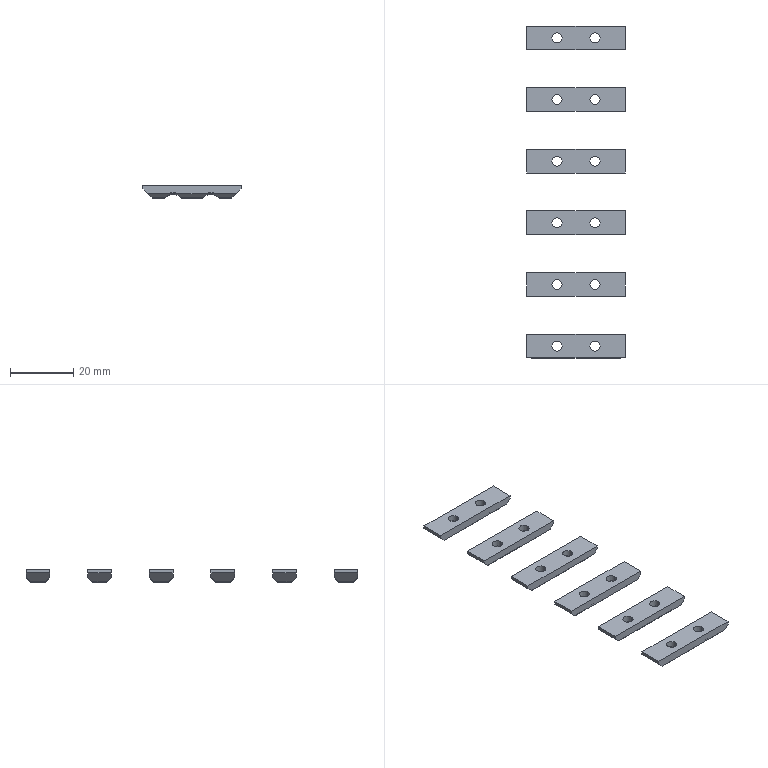NC program | NX | posted with a generic post | part box 31 x 105 x 4 mm
Whole program:
N10 G17 G21 G94 G90
(FLOOR_WALL_COPY_COPY , TOOL : D10JING)
N12 T14 M6
N14 G54
N16 G17 G0 G90 X-25.5 Y3.747 S51980 M3
N18 G43 Z30. H14
N20 Z6.
N22 G94 G1 Z3. F1500.
N24 X-20.5
N26 X20.5
N28 Y0.25
N30 X-20.5
N32 X-25.5
N34 Z6.
N36 G0 Z30.
N38 Y3.747
N40 Z5.
N42 G1 Z2.
N44 X-20.5
N46 X20.5
N48 Y0.25
N50 X-20.5
N52 X-25.5
N54 Z5.
N56 G0 Z30.
N58 Y3.747
N60 Z4.
N62 G1 Z1.
N64 X-20.5
N66 X20.5
N68 Y0.25
N70 X-20.5
N72 X-25.5
N74 Z4.
N76 G0 Z30.
N78 Y3.747
N80 Z3.
N82 G1 Z0.
N84 X-20.5
N86 X20.5
N88 Y0.25
N90 X-20.5
N92 X-25.5
N94 Z3.
N96 G0 Z30.
N98 M5
(PLANAR_MILL_COPY_COPY_COPY_COPY_COPY_COPY_1_COPY , TOOL : D6A45)
N100 T01 M6
N102 G54
N104 G17 G0 G90 X-5.567 Y0.45 S9500 M3
N106 G43 Z30. H1
N108 Z0.5
N110 G94 G1 Z-1. F1250.
N112 G3 X-6. Y0.7 R0.5
N114 X-6.7 Y0. R0.7
N116 X-6. Y0.7 R-0.7
N118 X-6.433 Y0.45 R0.5
N120 G1 Z0.5
N122 G0 Z30.
N124 X0.866 Y-5.15
N126 Z0.5
N128 G1 Z-1.
N130 G3 X0. Y-4.65 R1.
N132 G1 X-15.5
N134 G2 X-16.4 Y-3.75 R0.9
N136 G1 Y3.75
N138 G2 X-15.5 Y4.65 R0.9
N140 G1 X15.5
N142 G2 X16.4 Y3.75 R0.9
N144 G1 Y-3.75
N146 G2 X15.5 Y-4.65 R0.9
N148 G1 X0.
N150 G3 X-0.866 Y-5.15 R1.
N152 G1 Z0.5
N154 G0 Z30.
N156 X6.433 Y0.45
N158 Z0.5
N160 G1 Z-1.
N162 G3 X6. Y0.7 R0.5
N164 X5.3 Y0. R0.7
N166 X6. Y0.7 R-0.7
N168 X5.567 Y0.45 R0.5
N170 G1 Z0.5
N172 G0 Z30.
N174 M5
N176 M2